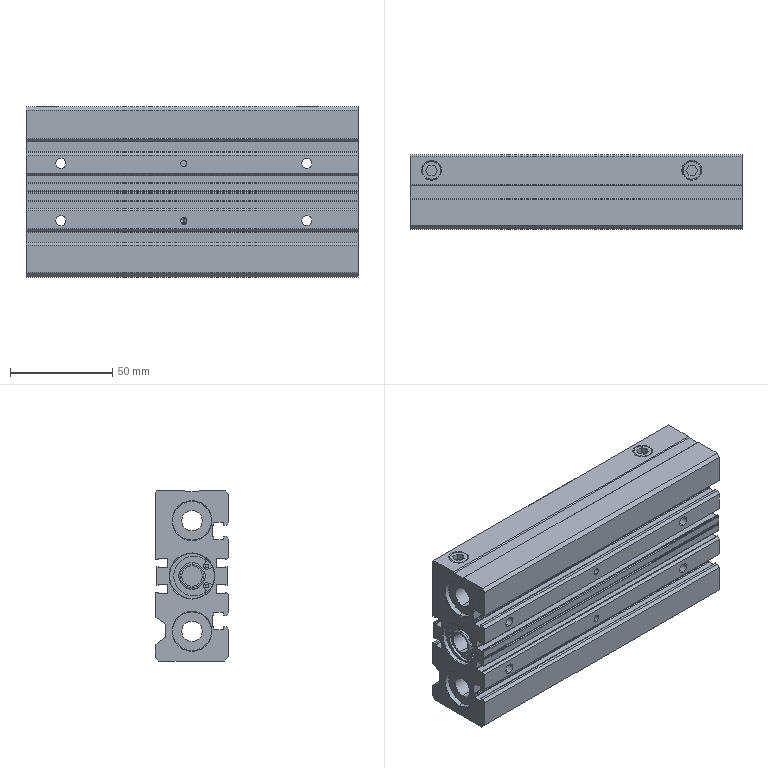Part | STEP file | TC-L-20x125125_b_HI | 1 solid | 389 faces | box 162 x 36 x 83 mm | volume 325855 mm3 | cylinder 186 | plane 139 | cone 62 | torus 2 | commonest cylinder face diameters 0.8 x20 0.4 x18 3 x14 1.8 x12 0.6 x10 1.5 x10